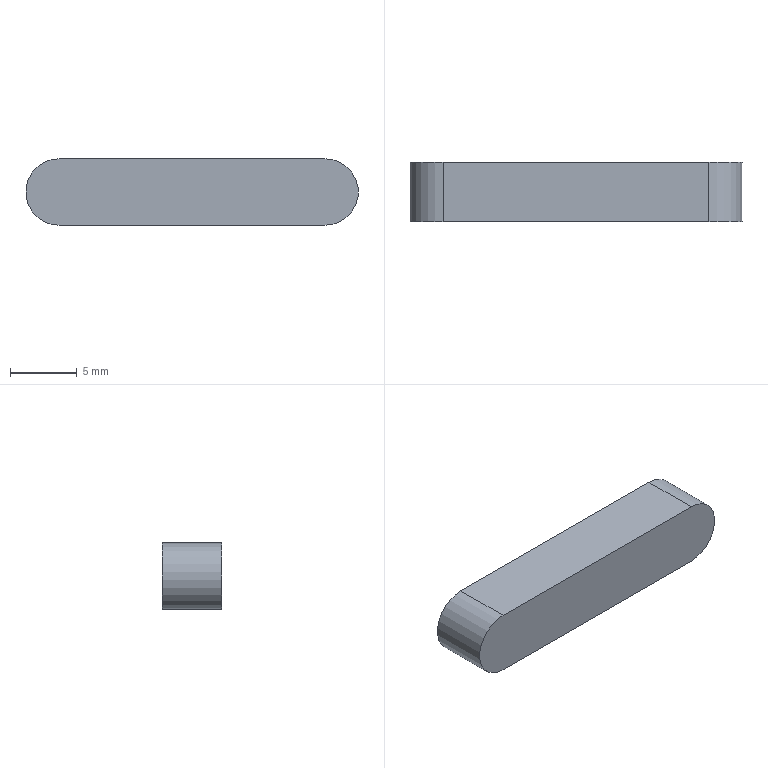Part | SolidWorks | features Extrusion 1 | 1 solid | 6 faces | box 25 x 4.5 x 5 mm | volume 538.357 mm3 | plane 4 | cylinder 2 | commonest cylinder face diameters 5 x2
STEP:
#1=CARTESIAN_POINT('',(-10.,0.,-2.5));
#2=VERTEX_POINT('',#1);
#3=CARTESIAN_POINT('',(-10.,0.,2.5));
#4=VERTEX_POINT('',#3);
#5=CARTESIAN_POINT('',(-10.,0.,0.));
#6=DIRECTION('',(0.,1.,0.));
#7=DIRECTION('',(0.,0.,-1.));
#8=AXIS2_PLACEMENT_3D('',#5,#6,#7);
#9=CIRCLE('',#8,2.5);
#10=EDGE_CURVE('',#2,#4,#9,.T.);
#11=ORIENTED_EDGE('',*,*,#10,.T.);
#12=CARTESIAN_POINT('',(-10.,4.5,2.5));
#13=VERTEX_POINT('',#12);
#14=CARTESIAN_POINT('',(-10.,4.5,2.5));
#15=DIRECTION('',(0.,-1.,0.));
#16=VECTOR('',#15,1000.);
#17=LINE('',#14,#16);
#18=EDGE_CURVE('',#13,#4,#17,.T.);
#19=ORIENTED_EDGE('',*,*,#18,.F.);
#20=CARTESIAN_POINT('',(-10.,4.5,-2.5));
#21=VERTEX_POINT('',#20);
#22=CARTESIAN_POINT('',(-10.,4.5,0.));
#23=DIRECTION('',(0.,1.,0.));
#24=DIRECTION('',(0.,0.,-1.));
#25=AXIS2_PLACEMENT_3D('',#22,#23,#24);
#26=CIRCLE('',#25,2.5);
#27=EDGE_CURVE('',#21,#13,#26,.T.);
#28=ORIENTED_EDGE('',*,*,#27,.F.);
#29=CARTESIAN_POINT('',(-10.,4.5,-2.5));
#30=DIRECTION('',(0.,-1.,0.));
#31=VECTOR('',#30,1000.);
#32=LINE('',#29,#31);
#33=EDGE_CURVE('',#21,#2,#32,.T.);
#34=ORIENTED_EDGE('',*,*,#33,.T.);
#35=EDGE_LOOP('',(#11,#19,#28,#34));
#36=FACE_OUTER_BOUND('',#35,.T.);
#37=CARTESIAN_POINT('',(-10.,4.5,0.));
#38=DIRECTION('',(0.,-1.,0.));
#39=DIRECTION('',(0.,0.,-1.));
#40=AXIS2_PLACEMENT_3D('',#37,#38,#39);
#41=CYLINDRICAL_SURFACE('',#40,2.5);
#42=ADVANCED_FACE('',(#36),#41,.T.);
#43=CARTESIAN_POINT('',(10.,0.,2.5));
#44=VERTEX_POINT('',#43);
#45=CARTESIAN_POINT('',(10.,0.,2.5));
#46=DIRECTION('',(1.,0.,0.));
#47=VECTOR('',#46,1000.);
#48=LINE('',#45,#47);
#49=EDGE_CURVE('',#4,#44,#48,.T.);
#50=ORIENTED_EDGE('',*,*,#49,.T.);
#51=CARTESIAN_POINT('',(10.,4.5,2.5));
#52=VERTEX_POINT('',#51);
#53=CARTESIAN_POINT('',(10.,4.5,2.5));
#54=DIRECTION('',(0.,-1.,0.));
#55=VECTOR('',#54,1000.);
#56=LINE('',#53,#55);
#57=EDGE_CURVE('',#52,#44,#56,.T.);
#58=ORIENTED_EDGE('',*,*,#57,.F.);
#59=CARTESIAN_POINT('',(10.,4.5,2.5));
#60=DIRECTION('',(1.,0.,0.));
#61=VECTOR('',#60,1000.);
#62=LINE('',#59,#61);
#63=EDGE_CURVE('',#13,#52,#62,.T.);
#64=ORIENTED_EDGE('',*,*,#63,.F.);
#65=ORIENTED_EDGE('',*,*,#18,.T.);
#66=EDGE_LOOP('',(#50,#58,#64,#65));
#67=FACE_OUTER_BOUND('',#66,.T.);
#68=CARTESIAN_POINT('',(10.,4.5,2.5));
#69=DIRECTION('',(0.,0.,-1.));
#70=DIRECTION('',(-1.,0.,0.));
#71=AXIS2_PLACEMENT_3D('',#68,#69,#70);
#72=PLANE('',#71);
#73=ADVANCED_FACE('',(#67),#72,.F.);
#74=CARTESIAN_POINT('',(10.,0.,-2.5));
#75=VERTEX_POINT('',#74);
#76=CARTESIAN_POINT('',(10.,0.,0.));
#77=DIRECTION('',(0.,1.,0.));
#78=DIRECTION('',(0.,0.,-1.));
#79=AXIS2_PLACEMENT_3D('',#76,#77,#78);
#80=CIRCLE('',#79,2.5);
#81=EDGE_CURVE('',#44,#75,#80,.T.);
#82=ORIENTED_EDGE('',*,*,#81,.T.);
#83=CARTESIAN_POINT('',(10.,4.5,-2.5));
#84=VERTEX_POINT('',#83);
#85=CARTESIAN_POINT('',(10.,4.5,-2.5));
#86=DIRECTION('',(0.,-1.,0.));
#87=VECTOR('',#86,1000.);
#88=LINE('',#85,#87);
#89=EDGE_CURVE('',#84,#75,#88,.T.);
#90=ORIENTED_EDGE('',*,*,#89,.F.);
#91=CARTESIAN_POINT('',(10.,4.5,0.));
#92=DIRECTION('',(0.,1.,0.));
#93=DIRECTION('',(0.,0.,-1.));
#94=AXIS2_PLACEMENT_3D('',#91,#92,#93);
#95=CIRCLE('',#94,2.5);
#96=EDGE_CURVE('',#52,#84,#95,.T.);
#97=ORIENTED_EDGE('',*,*,#96,.F.);
#98=ORIENTED_EDGE('',*,*,#57,.T.);
#99=EDGE_LOOP('',(#82,#90,#97,#98));
#100=FACE_OUTER_BOUND('',#99,.T.);
#101=CARTESIAN_POINT('',(10.,4.5,0.));
#102=DIRECTION('',(0.,-1.,0.));
#103=DIRECTION('',(0.,0.,-1.));
#104=AXIS2_PLACEMENT_3D('',#101,#102,#103);
#105=CYLINDRICAL_SURFACE('',#104,2.5);
#106=ADVANCED_FACE('',(#100),#105,.T.);
#107=CARTESIAN_POINT('',(-10.,0.,-2.5));
#108=DIRECTION('',(-1.,0.,0.));
#109=VECTOR('',#108,1000.);
#110=LINE('',#107,#109);
#111=EDGE_CURVE('',#75,#2,#110,.T.);
#112=ORIENTED_EDGE('',*,*,#111,.T.);
#113=ORIENTED_EDGE('',*,*,#33,.F.);
#114=CARTESIAN_POINT('',(-10.,4.5,-2.5));
#115=DIRECTION('',(-1.,0.,0.));
#116=VECTOR('',#115,1000.);
#117=LINE('',#114,#116);
#118=EDGE_CURVE('',#84,#21,#117,.T.);
#119=ORIENTED_EDGE('',*,*,#118,.F.);
#120=ORIENTED_EDGE('',*,*,#89,.T.);
#121=EDGE_LOOP('',(#112,#113,#119,#120));
#122=FACE_OUTER_BOUND('',#121,.T.);
#123=CARTESIAN_POINT('',(-10.,4.5,-2.5));
#124=DIRECTION('',(0.,0.,1.));
#125=DIRECTION('',(1.,0.,0.));
#126=AXIS2_PLACEMENT_3D('',#123,#124,#125);
#127=PLANE('',#126);
#128=ADVANCED_FACE('',(#122),#127,.F.);
#129=ORIENTED_EDGE('',*,*,#27,.T.);
#130=ORIENTED_EDGE('',*,*,#63,.T.);
#131=ORIENTED_EDGE('',*,*,#96,.T.);
#132=ORIENTED_EDGE('',*,*,#118,.T.);
#133=EDGE_LOOP('',(#129,#130,#131,#132));
#134=FACE_OUTER_BOUND('',#133,.T.);
#135=CARTESIAN_POINT('',(-10.,4.5,0.));
#136=DIRECTION('',(0.,-1.,0.));
#137=DIRECTION('',(0.,0.,-1.));
#138=AXIS2_PLACEMENT_3D('',#135,#136,#137);
#139=PLANE('',#138);
#140=ADVANCED_FACE('',(#134),#139,.F.);
#141=ORIENTED_EDGE('',*,*,#10,.F.);
#142=ORIENTED_EDGE('',*,*,#111,.F.);
#143=ORIENTED_EDGE('',*,*,#81,.F.);
#144=ORIENTED_EDGE('',*,*,#49,.F.);
#145=EDGE_LOOP('',(#141,#142,#143,#144));
#146=FACE_OUTER_BOUND('',#145,.T.);
#147=CARTESIAN_POINT('',(-10.,0.,0.));
#148=DIRECTION('',(0.,-1.,0.));
#149=DIRECTION('',(0.,0.,-1.));
#150=AXIS2_PLACEMENT_3D('',#147,#148,#149);
#151=PLANE('',#150);
#152=ADVANCED_FACE('',(#146),#151,.T.);
#153=CLOSED_SHELL('',(#42,#73,#106,#128,#140,#152));
#154=MANIFOLD_SOLID_BREP('',#153);
#155=CARTESIAN_POINT('',(0.,0.,0.));
#156=DIRECTION('',(0.,0.,1.));
#157=DIRECTION('',(1.,0.,0.));
#158=AXIS2_PLACEMENT_3D('',#155,#156,#157);
#159=(LENGTH_UNIT()NAMED_UNIT(*)SI_UNIT(.MILLI.,.METRE.));
#160=UNCERTAINTY_MEASURE_WITH_UNIT(LENGTH_MEASURE(0.00001),#159,'','');
#161=(NAMED_UNIT(*)PLANE_ANGLE_UNIT()SI_UNIT($,.RADIAN.));
#162=(NAMED_UNIT(*)SI_UNIT($,.STERADIAN.)SOLID_ANGLE_UNIT());
#163=(GEOMETRIC_REPRESENTATION_CONTEXT(3)GLOBAL_UNCERTAINTY_ASSIGNED_CONTEXT((#160))GLOBAL_UNIT_ASSIGNED_CONTEXT((#159,#161,#162))REPRESENTATION_CONTEXT('',''));
#164=ADVANCED_BREP_SHAPE_REPRESENTATION('',(#154,#158),#163);